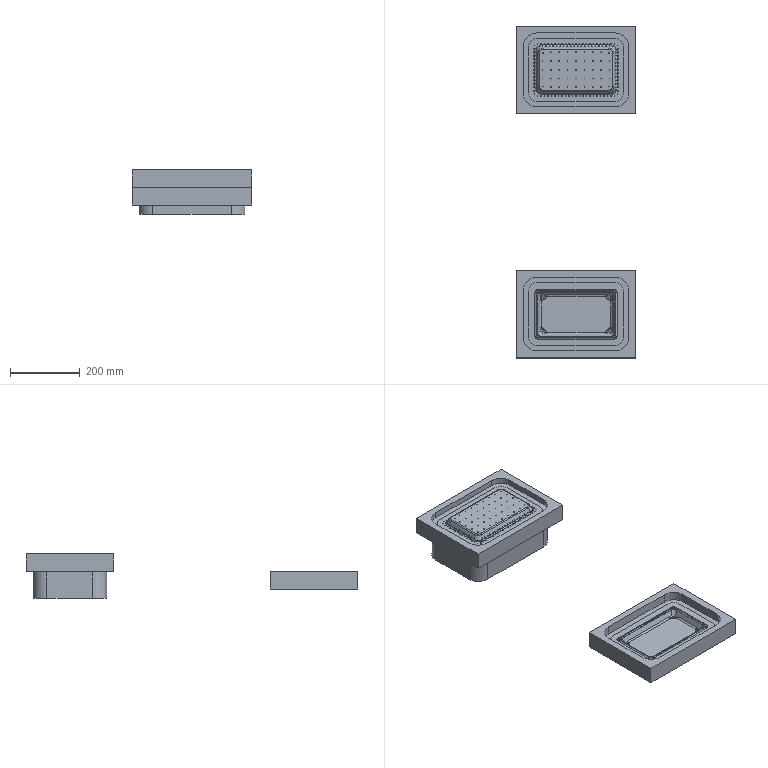NC program | NX | posted with a generic post | part box 343.99 x 952.259 x 127.368 mm
Lines 10630 to 11489 of 51088:
(CAVITY_MILL_4_COPY , TOOL : D4)
N21252 M6
N21254 G53
N21256 G17 G0 G90 X172.795 Y-251.657 S8000 M3 M8
N21258 G43 Z150. H0
N21260 Z-23.248
N21262 G94 G1 Z-24.248 F4000.
N21264 Y-247.95
N21266 G3 X171.995 Y-247.15 R0.8
N21268 G1 X284.407
N21270 G2 X321.84 Y-284.583 R37.433
N21272 G1 Y-416.546
N21274 G2 X284.407 Y-453.979 R37.433
N21276 G1 X59.583
N21278 G2 X22.15 Y-416.546 R37.433
N21280 G1 Y-284.583
N21282 G2 X59.583 Y-247.15 R37.433
N21284 G1 X171.995
N21286 Y-248.95
N21288 X284.407
N21290 G2 X320.04 Y-284.583 R35.633
N21292 G1 Y-416.546
N21294 G2 X284.407 Y-452.179 R35.633
N21296 G1 X59.583
N21298 G2 X23.95 Y-416.546 R35.633
N21300 G1 Y-284.583
N21302 G2 X59.583 Y-248.95 R35.633
N21304 G1 X171.995
N21306 G3 X172.795 Y-248.15 R0.8
N21308 G1 Y-251.657
N21310 Z-23.248
N21312 G0 Z3.
N21314 Z-23.493
N21316 G1 Z-24.493
N21318 Y-247.95
N21320 G3 X171.995 Y-247.15 R0.8
N21322 G1 X284.407
N21324 G2 X321.84 Y-284.583 R37.433
N21326 G1 Y-416.546
N21328 G2 X284.407 Y-453.979 R37.433
N21330 G1 X59.583
N21332 G2 X22.15 Y-416.546 R37.433
N21334 G1 Y-284.583
N21336 G2 X59.583 Y-247.15 R37.433
N21338 G1 X171.995
N21340 Y-248.95
N21342 X284.407
N21344 G2 X320.04 Y-284.583 R35.633
N21346 G1 Y-416.546
N21348 G2 X284.407 Y-452.179 R35.633
N21350 G1 X59.583
N21352 G2 X23.95 Y-416.546 R35.633
N21354 G1 Y-284.583
N21356 G2 X59.583 Y-248.95 R35.633
N21358 G1 X171.995
N21360 G3 X172.795 Y-248.15 R0.8
N21362 G1 Y-251.657
N21364 Z-23.493
N21366 G0 Z-21.248
N21368 X148.244 Y-247.15
N21370 Z-23.493
N21372 G1 X171.995 Z-24.738
N21374 X284.407
N21376 G2 X321.84 Y-284.583 R37.433
N21378 G1 Y-416.546
N21380 G2 X284.407 Y-453.979 R37.433
N21382 G1 X59.583
N21384 G2 X22.15 Y-416.546 R37.433
N21386 G1 Y-284.583
N21388 G2 X59.583 Y-247.15 R37.433
N21390 G1 X171.995
N21392 Y-248.95
N21394 X284.407
N21396 G2 X320.04 Y-284.583 R35.633
N21398 G1 Y-416.546
N21400 G2 X284.407 Y-452.179 R35.633
N21402 G1 X59.583
N21404 G2 X23.95 Y-416.546 R35.633
N21406 G1 Y-284.583
N21408 G2 X59.583 Y-248.95 R35.633
N21410 G1 X171.995
N21412 G3 X172.795 Y-248.15 R0.8
N21414 G1 Y-251.89
N21416 Z-23.738
N21418 G0 Z-21.493
N21420 X148.244 Y-247.15
N21422 Z-23.738
N21424 G1 X171.995 Z-24.982
N21426 X284.407
N21428 G2 X321.84 Y-284.583 R37.433
N21430 G1 Y-416.546
N21432 G2 X284.407 Y-453.979 R37.433
N21434 G1 X59.583
N21436 G2 X22.15 Y-416.546 R37.433
N21438 G1 Y-284.583
N21440 G2 X59.583 Y-247.15 R37.433
N21442 G1 X171.995
N21444 Y-248.95
N21446 X284.407
N21448 G2 X320.04 Y-284.583 R35.633
N21450 G1 Y-416.546
N21452 G2 X284.407 Y-452.179 R35.633
N21454 G1 X59.583
N21456 G2 X23.95 Y-416.546 R35.633
N21458 G1 Y-284.583
N21460 G2 X59.583 Y-248.95 R35.633
N21462 G1 X171.995
N21464 G3 X172.795 Y-248.15 R0.8
N21466 G1 Y-252.29
N21468 Z-23.982
N21470 G0 Z-19.29
N21472 X268.827 Y-301.293
N21474 Z-38.869
N21476 G1 Z-39.869
N21478 X270.11 Y-300.009
N21480 G3 X270.109 Y-298.878 R0.8
N21482 X268.698 Y-297.978 R3.888
N21484 G2 X267.411 Y-295.776 R2.
N21486 G1 X267.444
N21488 G2 X273.214 Y-301.52 R5.725
N21490 G1 Y-301.572
N21492 G2 X271.011 Y-300.288 R2.
N21494 G3 X270.109 Y-298.878 R3.888
N21496 X268.978 Y-298.879 R0.8
N21498 G1 X267.695 Y-300.162
N21500 Z-38.869
N21502 G0 Z-36.621
N21504 X268.703 Y-301.417
N21506 Z-39.117
N21508 G1 Z-40.117
N21510 X269.995 Y-300.124
N21512 G3 X269.994 Y-298.993 R0.8
N21514 X268.355 Y-298.017 R3.888
N21516 G2 X266.935 Y-295.891 R2.
N21518 G1 X267.383
N21520 G2 X273.099 Y-301.58 R5.702
N21522 G1 Y-302.055
N21524 G2 X270.973 Y-300.635 R2.
N21526 G3 X269.994 Y-298.993 R3.888
N21528 X268.863 Y-298.993 R0.8
N21530 G1 X267.571 Y-300.286
N21532 Z-39.117
N21534 G0 Z-36.869
N21536 X268.585 Y-301.536
N21538 Z-39.365
N21540 G1 Z-40.365
N21542 X269.88 Y-300.239
N21544 G3 X269.88 Y-299.107 R0.8
N21546 X267.84 Y-298.035 R3.888
N21548 G2 X266.204 Y-296.006 R2.
N21550 G1 X267.323
N21552 G2 X272.984 Y-301.641 R5.619
N21554 G1 Y-302.782
N21556 G2 X270.954 Y-301.148 R2.
N21558 G3 X269.88 Y-299.107 R3.888
N21560 X268.748 Y-299.108 R0.8
N21562 G1 X267.453 Y-300.405
N21564 Z-39.365
N21566 G0 Z-37.117
N21568 X268.47 Y-301.651
N21570 Z-39.613
N21572 G1 Z-40.613
N21574 X269.766 Y-300.353
N21576 G3 X269.765 Y-299.222 R0.8
N21578 X267.61 Y-298.13 R3.888
N21580 G2 X265.915 Y-296.12 R2.
N21582 G1 X267.263
N21584 G2 X272.87 Y-301.701 R5.564
N21586 G1 Y-303.072
N21588 G2 X270.859 Y-301.378 R2.
N21590 G3 X269.765 Y-299.222 R3.888
N21592 X268.634 Y-299.223 R0.8
N21594 G1 X267.338 Y-300.52
N21596 Z-39.613
N21598 G0 Z-37.365
N21600 X268.355 Y-301.765
N21602 Z-39.861
N21604 G1 Z-40.861
N21606 X269.651 Y-300.468
N21608 G3 X269.65 Y-299.337 R0.8
N21610 X267.428 Y-298.235 R3.888
N21612 G2 X265.698 Y-296.235 R2.
N21614 G1 X267.202
N21616 G2 X272.755 Y-301.762 R5.509
N21618 G1 Y-303.289
N21620 G2 X270.754 Y-301.56 R2.
N21622 G3 X269.65 Y-299.337 R3.888
N21624 X268.519 Y-299.337 R0.8
N21626 G1 X267.223 Y-300.634
N21628 Z-39.861
N21630 G0 Z-37.613
N21632 X268.24 Y-301.88
N21634 Z-40.109
N21636 G1 Z-41.109
N21638 X269.536 Y-300.583
N21640 G3 X269.536 Y-299.452 R0.8
N21642 X267.271 Y-298.344 R3.888
N21644 G2 X265.519 Y-296.35 R2.
N21646 G1 X267.142
N21648 G2 X272.64 Y-301.822 R5.454
N21650 G1 Y-303.469
N21652 G2 X270.645 Y-301.718 R2.
N21654 G3 X269.536 Y-299.452 R3.888
N21656 X268.404 Y-299.452 R0.8
N21658 G1 X267.109 Y-300.749
N21660 Z-40.109
N21662 G0 Z-37.861
N21664 X268.126 Y-301.995
N21666 Z-40.358
N21668 G1 Z-41.358
N21670 X269.422 Y-300.698
N21672 G3 X269.421 Y-299.566 R0.8
N21674 X267.145 Y-298.458 R3.888
N21676 G2 X265.388 Y-296.464 R2.
N21678 G1 X267.081
N21680 G2 X272.525 Y-301.883 R5.431
N21682 G1 Y-303.602
N21684 G2 X270.532 Y-301.845 R2.
N21686 G3 X269.421 Y-299.566 R3.888
N21688 X268.29 Y-299.567 R0.8
N21690 G1 X266.994 Y-300.864
N21692 Z-40.358
N21694 G0 Z-38.109
N21696 X268.011 Y-302.109
N21698 Z-40.606
N21700 G1 Z-41.606
N21702 X269.307 Y-300.812
N21704 G3 X269.307 Y-299.681 R0.8
N21706 X266.998 Y-298.569 R3.888
N21708 G2 X265.225 Y-296.579 R2.
N21710 G1 X267.021
N21712 G2 X272.411 Y-301.943 R5.346
N21714 G1 Y-303.764
N21716 G2 X270.421 Y-301.99 R2.
N21718 G3 X269.307 Y-299.681 R3.888
N21720 X268.175 Y-299.682 R0.8
N21722 G1 X266.879 Y-300.979
N21724 Z-40.606
N21726 G0 Z-38.358
N21728 X261.835 Y-301.058
N21730 Z-40.854
N21732 G1 Z-41.854
N21734 X261.198 Y-299.505
N21736 G3 X260.154 Y-299.068 R0.8
N21738 G1 X260.047 Y-299.115
N21740 X259.927 Y-299.168
N21742 X259.811 Y-299.222
N21744 G2 X257.104 Y-298.243 R2.
N21746 G3 X258.579 Y-297.672 R2.987
N21748 G1 X259.068 Y-297.331
N21750 G2 X261.643 Y-296.694 R5.524
N21752 G1 X263.084
N21754 G2 X261.378 Y-298.7 R2.
N21756 G3 X260.506 Y-298.936 R3.888
N21758 G1 X260.338 Y-298.999
N21760 X260.154 Y-299.068
N21762 G3 X259.718 Y-300.112 R0.8
N21764 G1 X260.327 Y-301.599
N21766 Z-40.854
N21768 G0 Z-38.606
N21770 X267.897 Y-302.224
N21772 Z-40.854
N21774 G1 Z-41.854
N21776 X269.193 Y-300.928
N21778 G3 X269.193 Y-299.797 R0.8
N21780 X266.874 Y-298.682 R3.888
N21782 G2 X265.096 Y-296.694 R2.
N21784 G1 X266.96
N21786 G2 X272.296 Y-302.004 R5.293
N21788 G1 Y-303.893
N21790 G2 X270.308 Y-302.114 R2.
N21792 G3 X269.193 Y-299.797 R3.888
N21794 X268.061 Y-299.797 R0.8
N21796 G1 X266.765 Y-301.093
N21798 Z-40.854
N21800 G0 Z-38.606
N21802 X267.548 Y-308.324
N21804 Z-40.854
N21806 G1 Z-41.854
N21808 X269.062 Y-308.885
N21810 G3 X270.09 Y-308.412 R0.8
N21812 X270.263 Y-307.791 R3.888
N21814 G2 X272.296 Y-306.167 R2.
N21816 G1 Y-307.096
N21818 G2 X271.787 Y-309.723 R6.374
N21820 G3 X270.805 Y-311.653 R4.085
N21822 G2 X269.858 Y-309.014 R2.
N21824 G3 X270.006 Y-308.643 R3.66
N21826 G1 X270.069 Y-308.467
N21828 X270.09 Y-308.412
N21830 G3 X269.617 Y-307.384 R0.8
N21832 G1 X268.044 Y-306.802
N21834 Z-40.854
N21836 G0 Z-38.606
N21838 X267.68 Y-305.552
N21840 Z-41.102
N21842 G1 Z-42.102
N21844 X269.28
N21846 G3 X270.08 Y-304.752 R0.8
N21848 G1 Y-302.57
N21850 G3 X266.42 Y-298.91 R3.66
N21852 G1 X262.055
N21854 G3 X259.916 Y-299.6 R3.66
N21856 G2 X256.978 Y-298.913 R2.
N21858 G3 X258.693 Y-298.037 R2.6
N21860 G2 X260.095 Y-297.133 R3.03
N21862 X262.252 Y-296.808 R7.592
N21864 G1 X266.903
N21866 G2 X271.297 Y-299.127 R5.286
N21868 X272.181 Y-302.062 R5.552
N21870 G1 Y-306.738
N21872 G2 X271.993 Y-308.482 R8.937
N21874 X270.923 Y-310.329 R3.608
N21876 G3 X270.082 Y-311.994 R2.662
N21878 G2 X269.39 Y-309.079 R2.
N21880 G3 X269.501 Y-308.912 R3.66
N21882 G1 X269.524 Y-308.875
N21884 G3 X270.08 Y-306.935 R3.66
N21886 G1 Y-304.752
N21888 G3 X269.28 Y-303.952 R0.8
N21890 G1 X267.68
N21892 Z-41.102
N21894 G0 Z-38.854
N21896 X267.219 Y-305.371
N21898 Z-41.35
N21900 G1 Z-42.35
N21902 X268.819
N21904 G3 X269.619 Y-304.571 R0.8
N21906 G1 Y-302.631
N21908 G3 X266.359 Y-299.371 R3.26
N21910 G1 X262.563
N21912 G3 X260.303 Y-300.282 R3.26
N21914 G1 X259.857 Y-300.711
N21916 X259.802 Y-300.763
N21918 X259.727 Y-300.832
N21920 G2 X256.6 Y-300.3 R2.
N21922 G1 X256.855
N21924 G3 X257.834 Y-299.936 R1.499
N21926 X258.511 Y-299.161 R3.661
N21928 G1 X259.068 Y-298.306
N21930 X259.122 Y-298.206
N21932 G2 X260.427 Y-297.227 R2.212
N21934 X262.382 Y-296.928 R8.789
N21936 G1 X266.879
N21938 G2 X268.074 Y-297.089 R8.183
N21940 X271.917 Y-300.988 R4.959
N21942 X272.062 Y-302.082 R8.944
N21944 G1 Y-306.655
N21946 G2 X271.298 Y-309.461 R5.037
N21948 G1 X271.053 Y-309.696
N21950 X269.86 Y-310.439
N21952 X269.83 Y-310.473
N21954 X269.306 Y-310.903
N21956 G3 X268.697 Y-312.053 R1.68
N21958 G2 X268.487 Y-308.988 R2.
N21960 G1 X268.508 Y-308.968
N21962 X268.634 Y-308.846
N21964 G3 X269.619 Y-306.511 R3.26
N21966 G1 Y-304.571
N21968 G3 X268.819 Y-303.771 R0.8
N21970 G1 X267.219
N21972 Z-41.35
N21974 G0 Z-39.102
N21976 X267.084 Y-297.076
N21978 Z-41.35
N21980 G1 X267.421 Y-297.081 Z-41.368
N21982 X268.722 Y-297.408 Z-41.438
N21984 X269.9 Y-298.05 Z-41.508
N21986 X270.319 Y-298.427 Z-41.538
N21988 X270.723 Y-298.815 Z-41.567
N21990 X271.517 Y-300.102 Z-41.646
N21992 X271.91 Y-301.563 Z-41.726
N21994 X271.917 Y-302.122 Z-41.755
N21996 Y-306.706 Z-41.995
N21998 X271.904 Y-307.241 Z-42.023
N22000 X271.562 Y-308.481 Z-42.091
N22002 X271.297 Y-308.948 Z-42.119
N22004 X271.17 Y-309.174 Z-42.132
N22006 X270.662 Y-309.494 Z-42.164
N22008 X270.061 Y-309.51 Z-42.195
N22010 X269.83 Y-309.393 Z-42.209
N22012 X268.76 Y-308.817 Z-42.273
N22014 X268.526 Y-308.673 Z-42.287
N22016 X266.526 Y-307.293 Z-42.414
N22018 X264.886 Y-305.92 Z-42.527
N22020 X264.031 Y-305.057 Z-42.59
N22022 X264.022 Y-305.048 Z-42.591
N22024 X264.013 Y-305.039
N22026 G2 X259.627 Y-299.185 R23.012
N22028 X260.046 Y-297.694 R1.073
N22030 X262.276 Y-297.073 R4.963
N22032 G1 X266.857
N22034 G2 X270.319 Y-298.427 R5.285
N22036 X271.917 Y-302.122 R5.205
N22038 G1 Y-306.706
N22040 G2 X271.297 Y-308.948 R4.772
N22042 X269.83 Y-309.393 R1.108
N22044 X264.031 Y-305.057 R24.581
N22046 G1 X264.013 Y-305.039
N22048 X265.958 Y-303.026
N22050 G2 X263.301 Y-299.873 R20.212
N22052 G1 X266.835
N22054 G2 X268.412 Y-300.478 R2.485
N22056 X269.117 Y-302.14 R2.405
N22058 G1 Y-305.678
N22060 G2 X265.997 Y-303.063 R21.781
N22062 G1 X265.958 Y-303.026
N22064 G3 X264.827 Y-303.045 R0.8
N22066 G1 Z-41.591
N22068 G0 Z-39.35
N22070 X263.674 Y-304.216
N22072 Z-41.591
N22074 G1 X262.303 Y-302.685 Z-41.699
N22076 X260.849 Y-300.675 Z-41.829
N22078 X260.582 Y-300.258 Z-41.855
N22080 X259.857 Y-298.963 Z-41.933
N22082 X259.85 Y-298.464 Z-41.959
N22084 X260.084 Y-298.022 Z-41.985
N22086 X260.69 Y-297.619 Z-42.023
N22088 X261.818 Y-297.256 Z-42.086
N22090 X262.302 Y-297.238 Z-42.111
N22092 X266.831 Z-42.348
N22094 X267.385 Y-297.242 Z-42.377
N22096 X268.753 Y-297.595 Z-42.451
N22098 X269.972 Y-298.308 Z-42.525
N22100 X270.368 Y-298.695 Z-42.554
N22102 X270.747 Y-299.089 Z-42.583
N22104 X271.421 Y-300.267 Z-42.654
N22106 X271.752 Y-301.584 Z-42.725
N22108 Y-303.638 Z-42.833
N22110 Y-306.525
N22112 G2 X271.203 Y-308.594 R4.493
N22114 X269.79 Y-309. R1.034
N22116 X259.976 Y-299.176 R25.636
N22118 X260.287 Y-297.888 R0.975
N22120 X262.302 Y-297.238 R3.901
N22122 G1 X266.831
N22124 G2 X270.368 Y-298.695 R5.104
N22126 X271.752 Y-302.13 R4.955
N22128 G1 Y-303.638
N22130 X268.952
N22132 Y-305.146
N22134 G2 X263.844 Y-300.038 R22.836
N22136 G1 X266.82
N22138 G2 X268.379 Y-300.667 R2.304
N22140 X268.952 Y-302.13 R2.155
N22142 G1 Y-303.638
N22144 G3 X269.752 Y-304.438 R0.8
N22146 G1 Z-41.833
N22148 G0 Z-39.591
N22150 X264.56 Y-304.77
N22152 Z-41.833
N22154 G1 X264.383 Y-304.607 Z-41.846
N22156 X262.839 Y-302.925 Z-41.965
N22158 X261.318 Y-300.928 Z-42.097
N22160 X261.043 Y-300.521 Z-42.123
N22162 X260.261 Y-299.207 Z-42.203
N22164 X260.251 Y-298.445 Z-42.243
N22166 X260.384 Y-298.206 Z-42.257
N22168 X260.694 Y-297.921 Z-42.279
N22170 X261.278 Y-297.61 Z-42.314
N22172 X261.915 Y-297.435 Z-42.348
N22174 X262.337 Y-297.43 Z-42.37
N22176 X266.829 Z-42.606
N22178 X266.895 Y-297.46 Z-42.61
N22180 X267.421 Y-297.455 Z-42.637
N22182 X268.778 Y-297.81 Z-42.711
N22184 X269.967 Y-298.557 Z-42.784
N22186 X270.876 Y-299.626 Z-42.858
N22188 X271.423 Y-300.918 Z-42.931
N22190 X271.572 Y-302.022 Z-42.99
N22192 X271.56 Y-302.61 Z-43.021
N22194 Y-303.638 Z-43.074
N22196 Y-306.714
N22198 G2 X271.145 Y-308.168 R4.813
N22200 X269.638 Y-308.637 R1.066
N22202 X260.401 Y-299.442 R26.247
N22204 X260.384 Y-298.206 R1.237
N22206 X262.337 Y-297.43 R2.943
N22208 G1 X266.829
N22210 X266.895 Y-297.46
N22212 G2 X271.494 Y-301.439 R4.594
N22214 X271.56 Y-302.61 R7.579
N22216 G1 Y-303.638
N22218 X268.76
N22220 Y-304.681
N22222 G2 X264.306 Y-300.23 R23.447
N22224 G1 X266.484
N22226 G3 X266.923 Y-300.26 R2.8
N22228 G2 X268.719 Y-301.814 R1.794
N22230 X268.76 Y-302.581 R4.779
N22232 G1 Y-303.638
N22234 G3 X269.56 Y-304.438 R0.8
N22236 G1 Z-42.074
N22238 G0 Z-39.833
N22240 X265.495 Y-305.278
N22242 Z-42.074
N22244 G1 X263.4 Y-303.184 Z-42.23
N22246 X261.83 Y-301.216 Z-42.362
N22248 X261.497 Y-300.743 Z-42.392
N22250 X260.832 Y-299.674 Z-42.458
N22252 X260.608 Y-299.185 Z-42.486
N22254 X260.518 Y-298.971 Z-42.498
N22256 X260.527 Y-298.659 Z-42.515
N22258 X260.629 Y-298.451 Z-42.527
N22260 X260.853 Y-298.171 Z-42.546
N22262 X261.349 Y-297.839 Z-42.577
N22264 X261.918 Y-297.656 Z-42.608
N22266 X262.276 Y-297.654 Z-42.627
N22268 X266.895 Z-42.869
N22270 X267.414 Y-297.658 Z-42.896
N22272 X268.574 Y-297.964 Z-42.959
N22274 X269.612 Y-298.565 Z-43.022
N22276 X270.455 Y-299.418 Z-43.085
N22278 X271.044 Y-300.463 Z-43.148
N22280 X271.336 Y-301.626 Z-43.211
N22282 X271.334 Y-302.145 Z-43.238
N22284 X271.336 Y-302.61 Z-43.262
N22286 Y-303.638 Z-43.316
N22288 Y-306.644
N22290 G2 X270.564 Y-308.346 R2.262
N22292 X269.46 Y-308.247 R1.248
N22294 X260.832 Y-299.674 R26.389
N22296 G1 X260.608 Y-299.185
N22298 G2 X260.629 Y-298.451 R0.885
N22300 X262.276 Y-297.654 R2.123
N22302 G1 X266.895
N22304 G2 X271.334 Y-302.145 R4.48
N22306 G1 X271.336 Y-302.61
N22308 Y-303.638
N22310 X268.536
N22312 Y-304.186
N22314 G2 X264.804 Y-300.454 R23.589
N22316 G1 X266.879
N22318 G2 X268.534 Y-302.148 R1.68
N22320 G1 X268.536 Y-302.616
N22322 Y-303.638
N22324 G3 X269.336 Y-304.438 R0.8
N22326 G1 Z-42.316
N22328 G0 Z-40.074
N22330 X262.922 Y-297.918
N22332 Z-42.316
N22334 G1 X266.833 Z-42.521
N22336 X267.338 Z-42.547
N22338 X268.697 Y-298.315 Z-42.622
N22340 X269.85 Y-299.135 Z-42.696
N22342 X270.672 Y-300.287 Z-42.77
N22344 X271.071 Y-301.645 Z-42.844
N22346 X271.072 Y-302.15 Z-42.871
N22348 Y-306.584 Z-43.103
N22350 X271.044 Y-307.02 Z-43.126
N22352 X271.027 Y-307.095 Z-43.13
N22354 X270.872 Y-307.503 Z-43.153
N22356 X270.792 Y-307.725 Z-43.165
N22358 X270.328 Y-308.078 Z-43.196
N22360 X269.745 Y-308.09 Z-43.226
N22362 X269.544 Y-307.967 Z-43.239
N22364 X268.48 Y-307.312 Z-43.304
N22366 X267.434 Y-306.56 Z-43.372
N22368 X265.594 Y-305.021 Z-43.497
N22370 X264.781 Y-304.209 Z-43.557
N22372 G2 X261.025 Y-299.462 R26.011
N22374 X261.321 Y-298.206 R0.909
N22376 G1 X261.514 Y-298.107
N22378 X262.37 Y-297.918
N22380 X266.833
N22382 G2 X271.072 Y-302.15 R4.235
N22384 G1 Y-306.584
N22386 G2 X270.872 Y-307.503 R3.165
N22388 X269.544 Y-307.967 R0.908
N22390 X264.781 Y-304.209 R26.011
N22392 G1 X266.76 Y-302.228
N22394 G2 X265.376 Y-300.718 R23.211
N22396 G1 X266.835
N22398 G2 X268.272 Y-302.151 R1.435
N22400 G1 Y-303.61
N22402 G2 X266.76 Y-302.228 R23.211
N22404 G3 X265.629 Y-302.229 R0.8
N22406 G1 Z-42.557
N22408 G0 Z-40.316
N22410 X261.653 Y-298.416
N22412 Z-42.557
N22414 G1 X261.934 Y-298.237 Z-42.575
N22416 X266.79 Z-42.829
N22418 X267.277 Y-298.234 Z-42.855
N22420 X268.533 Y-298.598 Z-42.923
N22422 X269.603 Y-299.351 Z-42.992
N22424 X270.37 Y-300.412 Z-43.061
N22426 X270.75 Y-301.663 Z-43.129
N22428 X270.753 Y-302.15 Z-43.155
N22430 Y-306.652 Z-43.391
N22432 X270.76 Y-306.933 Z-43.405
N22434 X270.529 Y-307.47 Z-43.436
N22436 X270.319 Y-307.658 Z-43.451
N22438 X270.096 Y-307.743 Z-43.463
N22440 X269.681 Y-307.701 Z-43.485
N22442 X268.415 Y-306.89 Z-43.564
N22444 X267.029 Y-305.837 Z-43.655
N22446 X265.535 Y-304.501 Z-43.76
N22448 X265.012 Y-303.978 Z-43.799
N22450 G2 X261.48 Y-299.609 R26.648
N22452 X261.264 Y-298.823 R1.349
N22454 X262.183 Y-298.237 R1.013
N22456 G1 X266.79
N22458 G2 X270.753 Y-302.15 R3.939
N22460 G1 Y-306.652
N22462 G2 X270.319 Y-307.658 R1.306
N22464 X269.48 Y-307.572 R0.935
N22466 X265.012 Y-303.978 R26.648
N22468 G1 X266.992 Y-301.998
N22470 G2 X266.083 Y-301.037 R23.848
N22472 G1 X266.807
N22474 G2 X267.953 Y-302.162 R1.139
N22476 G1 Y-302.907
N22478 G2 X266.992 Y-301.998 R23.848
N22480 G3 X265.861 Y-301.998 R0.8
N22482 G1 Z-42.799
N22484 G0 Z-40.557
N22486 X262.333 Y-300.191
N22488 Z-42.799
N22490 G1 X261.652 Y-299.112 Z-42.866
N22492 X261.648 Y-298.979 Z-42.873
N22494 X261.8 Y-298.704 Z-42.889
N22496 X261.915 Y-298.636 Z-42.896
N22498 X266.792 Z-43.152
N22500 X267.254 Y-298.633 Z-43.176
N22502 X267.389 Y-298.652 Z-43.183
N22504 X268.274 Y-298.917 Z-43.232
N22506 X269.339 Y-299.651 Z-43.299
N22508 X270.073 Y-300.717 Z-43.367
N22510 X270.338 Y-301.601 Z-43.416
N22512 X270.351 Y-301.686 Z-43.42
N22514 X270.354 Y-302.148 Z-43.444
N22516 Y-307.07 Z-43.702
N22518 X270.285 Y-307.187 Z-43.709
N22520 X270.008 Y-307.339 Z-43.726
N22522 X269.872 Y-307.335 Z-43.733
N22524 X268.688 Y-306.587 Z-43.807
N22526 X266.465 Y-304.837 Z-43.955
N22528 X265.433 Y-303.835 Z-44.03
N22530 X265.294 Y-303.696 Z-44.04
N22532 G2 X261.736 Y-299.245 R25.727
N22534 X262.072 Y-298.636 R0.397
N22536 G1 X266.792
N22538 G2 X270.354 Y-302.148 R3.537
N22540 G1 Y-306.912
N22542 G2 X269.738 Y-307.251 R0.401
N22544 X265.294 Y-303.696 R25.727
N22546 G1 X267.274 Y-301.716
N22548 G2 X267.028 Y-301.467 R22.927
N22550 X267.523 Y-301.962 R0.737
N22552 X267.274 Y-301.716 R22.927
N22554 G3 X266.142 Y-301.716 R0.8
N22556 G1 Z-43.04
N22558 G0 Z-40.799
N22560 X265.239 Y-302.859
N22562 Z-43.04
N22564 G1 X264.806 Y-302.426 Z-43.073
N22566 X263.018 Y-300.224 Z-43.221
N22568 X262.338 Y-299.184 Z-43.286
N22570 X267.236 Z-43.543
N22572 X268.163 Y-299.472 Z-43.594
N22574 X268.95 Y-300.04 Z-43.645
N22576 X269.518 Y-300.827 Z-43.696
N22578 X269.806 Y-301.754 Z-43.747
N22580 Y-306.65 Z-44.003
N22582 X268.766 Y-305.97 Z-44.068
N22584 X266.565 Y-304.183 Z-44.217
N22586 X265.686 Y-303.304 Z-44.282
N22588 G2 X262.338 Y-299.184 R25.739
N22590 G1 X266.811
N22592 G2 X269.806 Y-302.179 R2.995
N22594 G1 Y-306.65
N22596 G2 X265.686 Y-303.304 R25.739
N22598 G1 X266.958 Y-302.031
N22600 G2 X265.971 Y-300.984 R23.939
N22602 G1 X266.811
N22604 G2 X268.006 Y-302.179 R1.195
N22606 G1 Y-303.018
N22608 G2 X266.958 Y-302.031 R23.939
N22610 G3 X265.827 Y-302.032 R0.8
N22612 G1 Z-43.282
N22614 G0 Z-41.04
N22616 X267.777 Y-300.716
N22618 Z-43.282
N22620 G1 X268.095 Y-300.932 Z-43.302
N22622 X268.385 Y-301.342 Z-43.328
N22624 X268.661 Y-302.524 Z-43.392
N22626 Y-304.324 Z-43.486
N22628 X267.71 Y-303.571 Z-43.55
N22630 X265.417 Y-301.279 Z-43.72
N22632 X264.663 Y-300.328 Z-43.784
N22634 X266.182 Z-43.863
N22636 X267.68 Y-300.65 Z-43.943
N22638 X268.095 Y-300.932 Z-43.97
N22640 X268.385 Y-301.342 Z-43.996
N22642 X268.661 Y-302.524 Z-44.06
N22644 Y-304.324 Z-44.154
N22646 X267.71 Y-303.571 Z-44.218
N22648 X265.417 Y-301.279 Z-44.387
N22650 X264.663 Y-300.328 Z-44.451
N22652 X266.044 Z-44.523
N22654 X266.182
N22656 X267.398 Y-300.589
N22658 G2 X268.451 Y-301.624 R1.379
N22660 G1 X268.661 Y-302.524
N22662 Y-304.324
N22664 G2 X264.663 Y-300.328 R24.523
N22666 G1 X266.044
N22668 G3 X265.644 Y-300.728 R0.4
N22670 G1 Z-43.523
N22672 G0 Z-36.621
N22674 X268.264 Y-400.684
N22676 Z-38.869
N22678 G1 Z-39.869
N22680 X269.986 Y-401.314
N22682 G3 X271.012 Y-400.837 R0.8
N22684 G2 X273.214 Y-399.551 R2.
N22686 G1 Y-399.583
N22688 G2 X267.463 Y-405.353 R5.725
N22690 G1 X267.417
N22692 G2 X268.701 Y-403.15 R2.
N22694 G3 X271.012 Y-400.838 R3.888
N22696 X270.536 Y-399.811 R0.8
N22698 G1 X269.102 Y-399.286
N22700 Z-38.869
N22702 G0 Z-36.621
N22704 X268.129 Y-400.584
N22706 Z-39.117
N22708 G1 Z-40.117
N22710 X269.84 Y-401.243
N22712 G3 X270.874 Y-400.784 R0.8
N22714 X271.026 Y-400.297 R3.888
N22716 G2 X273.099 Y-398.77 R2.
N22718 G1 Y-399.523
N22720 G2 X267.403 Y-405.238 R5.673
N22722 G1 X266.634
N22724 G2 X268.16 Y-403.165 R2.
N22726 G3 X270.874 Y-400.784 R3.888
N22728 X270.416 Y-399.75 R0.8
N22730 G1 X268.875 Y-399.157
N22732 Z-39.117
N22734 G0 Z-36.869
N22736 X267.995 Y-400.483
N22738 Z-39.365
N22740 G1 Z-40.365
N22742 X269.695 Y-401.17
N22744 G3 X270.736 Y-400.728 R0.8
N22746 X270.955 Y-399.976 R3.888
N22748 G2 X272.984 Y-398.339 R2.
N22750 G1 Y-399.462
N22752 G2 X267.342 Y-405.124 R5.618
N22754 G1 X266.202
N22756 G2 X267.838 Y-403.095 R2.
N22758 G3 X270.736 Y-400.728 R3.888
N22760 X270.295 Y-399.687 R0.8
N22762 G1 X268.716 Y-399.049
N22764 Z-39.365
N22766 G0 Z-37.117
N22768 X267.861 Y-400.382
N22770 Z-39.613
N22772 G1 Z-40.613
N22774 X269.55 Y-401.096
N22776 G3 X270.598 Y-400.67 R0.8
N22778 X270.86 Y-399.748 R3.888
N22780 G2 X272.87 Y-398.052 R2.
N22782 G1 Y-399.402
N22784 G2 X267.281 Y-405.009 R5.562
N22786 G1 X265.915
N22788 G2 X267.61 Y-402.999 R2.
N22790 G3 X270.598 Y-400.67 R3.888
N22792 X270.173 Y-399.622 R0.8
N22794 G1 X268.577 Y-398.948
N22796 Z-39.613
N22798 G0 Z-37.365
N22800 X267.728 Y-400.28
N22802 Z-39.861
N22804 G1 Z-40.861
N22806 X269.406 Y-401.019
N22808 G3 X270.461 Y-400.609 R0.8
N22810 X270.755 Y-399.567 R3.888
N22812 G2 X272.755 Y-397.836 R2.
N22814 G1 Y-399.341
N22816 G2 X267.22 Y-404.894 R5.508
N22818 G1 X265.699
N22820 G2 X267.428 Y-402.894 R2.
N22822 G3 X270.461 Y-400.609 R3.888
N22824 X270.051 Y-399.555 R0.8
N22826 G1 X268.449 Y-398.849
N22828 Z-39.861
N22830 G0 Z-37.613
N22832 X267.595 Y-400.177
N22834 Z-40.109
N22836 G1 Z-41.109
N22838 X269.262 Y-400.94
N22840 G3 X270.323 Y-400.546 R0.8
N22842 X270.646 Y-399.409 R3.888
N22844 G2 X272.64 Y-397.657 R2.
N22846 G1 Y-399.281
N22848 G2 X267.16 Y-404.78 R5.453
N22850 G1 X265.52
N22852 G2 X267.271 Y-402.785 R2.
N22854 G3 X270.323 Y-400.546 R3.888
N22856 X269.928 Y-399.486 R0.8
N22858 G1 X268.325 Y-398.751
N22860 Z-40.109
N22862 G0 Z-37.861
N22864 X267.463 Y-400.074
N22866 Z-40.358
N22868 G1 Z-41.358
N22870 X269.119 Y-400.86
N22872 G3 X270.185 Y-400.481 R0.8
N22874 X270.534 Y-399.269 R3.888
N22876 G2 X272.525 Y-397.503 R2.
N22878 G1 Y-399.22
N22880 G2 X267.099 Y-404.665 R5.4
N22882 G1 X265.365
N22884 G2 X267.13 Y-402.673 R2.
N22886 G3 X270.185 Y-400.481 R3.888
N22888 X269.806 Y-399.415 R0.8
N22890 G1 X268.203 Y-398.654
N22892 Z-40.358
N22894 G0 Z-38.109
N22896 X267.331 Y-399.969
N22898 Z-40.606
N22900 G1 Z-41.606
N22902 X268.977 Y-400.778
N22904 G3 X270.048 Y-400.413 R0.8
N22906 X270.421 Y-399.137 R3.888
N22908 G2 X272.411 Y-397.363 R2.
N22910 G1 Y-399.16
N22912 G2 X267.039 Y-404.55 R5.345
N22914 G1 X265.225
N22916 G2 X266.999 Y-402.561 R2.
N22918 G3 X270.048 Y-400.413 R3.888
N22920 X269.683 Y-399.342 R0.8
N22922 G1 X268.083 Y-398.556
N22924 Z-40.606
N22926 G0 Z-38.358
N22928 X268.044 Y-394.331
N22930 Z-40.854
N22932 G1 Z-41.854
N22934 X269.615 Y-393.738
N22936 G3 X270.081 Y-392.707 R0.8
N22938 G1 X270.045 Y-392.614
N22940 X269.982 Y-392.45
N22942 G3 X269.836 Y-392.1 R3.66
N22944 G2 X270.795 Y-389.423 R2.
N22946 G3 X271.787 Y-391.407 R4.133
N22948 G2 X272.296 Y-394.026 R6.493
N22950 G1 Y-394.954
N22952 G2 X270.26 Y-393.337 R2.
N22954 G3 X270.081 Y-392.707 R3.888
N22956 X269.05 Y-392.241 R0.8
N22958 G1 X267.533 Y-392.814
N22960 Z-40.854
N22962 G0 Z-38.606
N22964 X267.602 Y-399.517